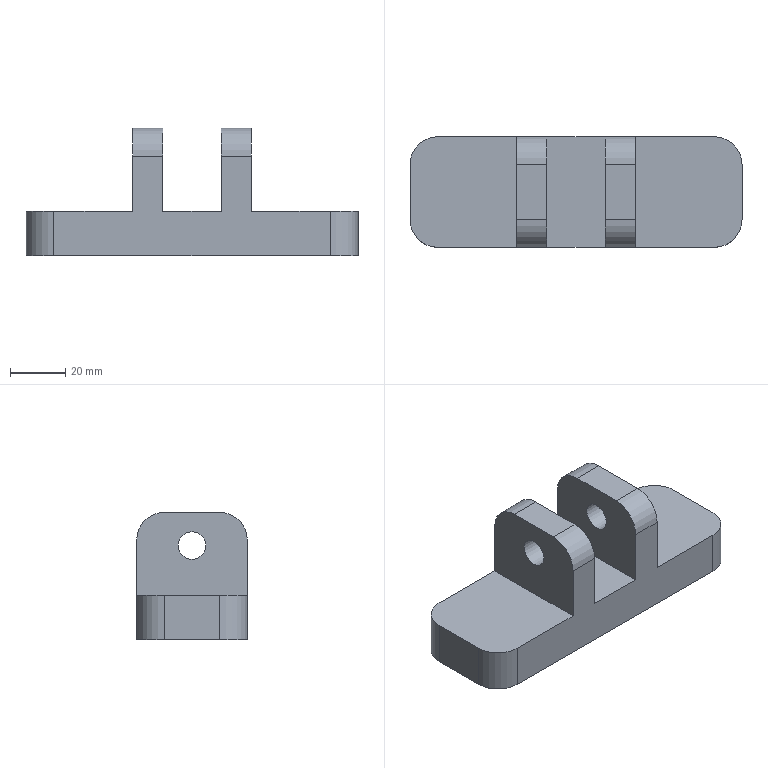NC program | NX | posted with a generic post | part box 120 x 40 x 46 mm
Lines 1 to 18 of 19901:
N10 G17 G21 G94 G90
(PLANAR_MILL , TOOL : D50面刀)
N12 T01 M6
N14 G53
N16 G17 G0 G90 X80. Y0. S1600 M3
N18 G43 Z20. H1
N20 Z2.
N22 G94 G1 Z0. F600.
N24 X50.
N26 X-50.
N28 X-80.
N30 Z2.
N32 G0 Z20.
N34 M5